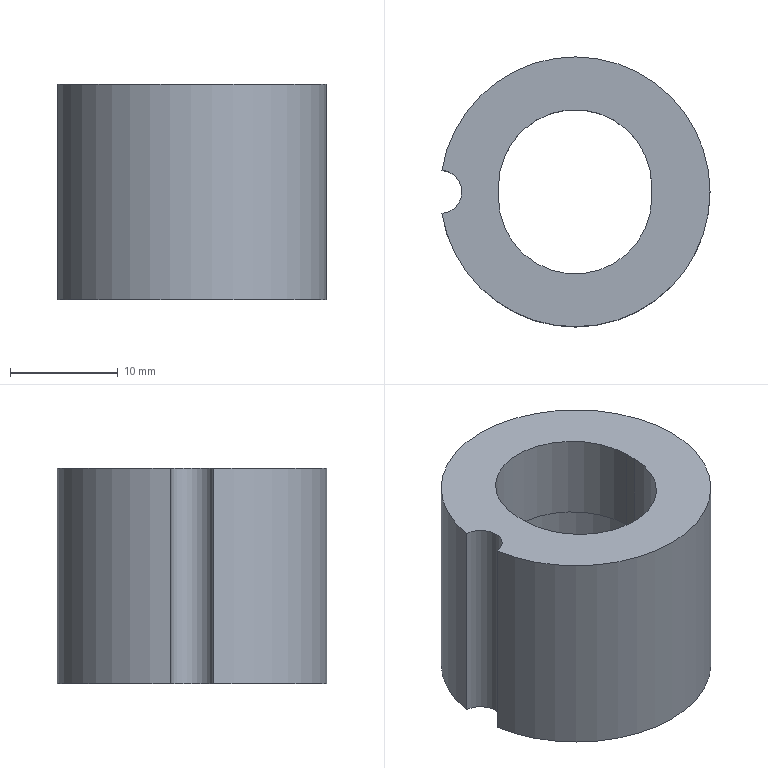Part | NX | features solid 2 | 1 solid | 10 faces | box 24.84 x 25 x 20 mm | volume 5715 mm3 | plane 5 | cylinder 5 | commonest cylinder face diameters 14.22 x2 4 x1 16.6 x1 25 x1
STEP:
#1=CARTESIAN_POINT('',(-114.371,25.823,-5.379));
#2=VERTEX_POINT('',#1);
#3=CARTESIAN_POINT('',(-114.371,21.836,-5.379));
#4=VERTEX_POINT('',#3);
#5=CARTESIAN_POINT('',(-114.531,23.83,-5.379));
#6=DIRECTION('',(0.,0.,-1.));
#7=DIRECTION('',(1.,0.,0.));
#8=AXIS2_PLACEMENT_3D('',#5,#6,#7);
#9=CIRCLE('',#8,2.);
#10=EDGE_CURVE('',#2,#4,#9,.T.);
#11=ORIENTED_EDGE('',*,*,#10,.T.);
#12=CARTESIAN_POINT('',(-102.031,23.83,-5.379));
#13=DIRECTION('',(0.,0.,1.));
#14=DIRECTION('',(-1.,0.,0.));
#15=AXIS2_PLACEMENT_3D('',#12,#13,#14);
#16=CIRCLE('',#15,12.5);
#17=EDGE_CURVE('',#2,#4,#16,.F.);
#18=ORIENTED_EDGE('',*,*,#17,.F.);
#19=EDGE_LOOP('',(#11,#18));
#20=FACE_BOUND('',#19,.T.);
#21=CARTESIAN_POINT('',(-94.921,23.33,-5.379));
#22=VERTEX_POINT('',#21);
#23=CARTESIAN_POINT('',(-109.141,23.33,-5.379));
#24=VERTEX_POINT('',#23);
#25=CARTESIAN_POINT('',(-102.031,23.33,-5.379));
#26=DIRECTION('',(0.,0.,-1.));
#27=DIRECTION('',(1.,0.,0.));
#28=AXIS2_PLACEMENT_3D('',#25,#26,#27);
#29=CIRCLE('',#28,7.11);
#30=EDGE_CURVE('',#22,#24,#29,.T.);
#31=ORIENTED_EDGE('',*,*,#30,.T.);
#32=CARTESIAN_POINT('',(-109.141,24.33,-5.379));
#33=VERTEX_POINT('',#32);
#34=CARTESIAN_POINT('',(-109.141,23.83,-5.379));
#35=DIRECTION('',(0.,1.,0.));
#36=VECTOR('',#35,1000.);
#37=LINE('',#34,#36);
#38=EDGE_CURVE('',#24,#33,#37,.T.);
#39=ORIENTED_EDGE('',*,*,#38,.T.);
#40=CARTESIAN_POINT('',(-94.921,24.33,-5.379));
#41=VERTEX_POINT('',#40);
#42=CARTESIAN_POINT('',(-102.031,24.33,-5.379));
#43=DIRECTION('',(0.,0.,-1.));
#44=DIRECTION('',(1.,0.,0.));
#45=AXIS2_PLACEMENT_3D('',#42,#43,#44);
#46=CIRCLE('',#45,7.11);
#47=EDGE_CURVE('',#33,#41,#46,.T.);
#48=ORIENTED_EDGE('',*,*,#47,.T.);
#49=CARTESIAN_POINT('',(-94.921,23.83,-5.379));
#50=DIRECTION('',(0.,-1.,0.));
#51=VECTOR('',#50,1000.);
#52=LINE('',#49,#51);
#53=EDGE_CURVE('',#41,#22,#52,.T.);
#54=ORIENTED_EDGE('',*,*,#53,.T.);
#55=EDGE_LOOP('',(#31,#39,#48,#54));
#56=FACE_BOUND('',#55,.T.);
#57=CARTESIAN_POINT('',(-102.031,23.83,-5.379));
#58=DIRECTION('',(0.,0.,1.));
#59=DIRECTION('',(-1.,0.,0.));
#60=AXIS2_PLACEMENT_3D('',#57,#58,#59);
#61=PLANE('',#60);
#62=ADVANCED_FACE('',(#20,#56),#61,.T.);
#63=CARTESIAN_POINT('',(-114.371,21.836,-25.379));
#64=VERTEX_POINT('',#63);
#65=CARTESIAN_POINT('',(-114.371,25.823,-25.379));
#66=VERTEX_POINT('',#65);
#67=CARTESIAN_POINT('',(-114.531,23.83,-25.379));
#68=DIRECTION('',(0.,0.,1.));
#69=DIRECTION('',(-1.,0.,0.));
#70=AXIS2_PLACEMENT_3D('',#67,#68,#69);
#71=CIRCLE('',#70,2.);
#72=EDGE_CURVE('',#64,#66,#71,.T.);
#73=ORIENTED_EDGE('',*,*,#72,.T.);
#74=CARTESIAN_POINT('',(-102.031,23.83,-25.379));
#75=DIRECTION('',(0.,0.,-1.));
#76=DIRECTION('',(1.,0.,0.));
#77=AXIS2_PLACEMENT_3D('',#74,#75,#76);
#78=CIRCLE('',#77,12.5);
#79=EDGE_CURVE('',#64,#66,#78,.F.);
#80=ORIENTED_EDGE('',*,*,#79,.F.);
#81=EDGE_LOOP('',(#73,#80));
#82=FACE_BOUND('',#81,.T.);
#83=CARTESIAN_POINT('',(-93.731,23.83,-25.379));
#84=VERTEX_POINT('',#83);
#85=CARTESIAN_POINT('',(-102.031,23.83,-25.379));
#86=DIRECTION('',(0.,0.,-1.));
#87=DIRECTION('',(1.,0.,0.));
#88=AXIS2_PLACEMENT_3D('',#85,#86,#87);
#89=CIRCLE('',#88,8.3);
#90=EDGE_CURVE('',#84,#84,#89,.F.);
#91=ORIENTED_EDGE('',*,*,#90,.T.);
#92=EDGE_LOOP('',(#91));
#93=FACE_BOUND('',#92,.T.);
#94=CARTESIAN_POINT('',(-102.031,23.83,-25.379));
#95=DIRECTION('',(0.,0.,-1.));
#96=DIRECTION('',(1.,0.,0.));
#97=AXIS2_PLACEMENT_3D('',#94,#95,#96);
#98=PLANE('',#97);
#99=ADVANCED_FACE('',(#82,#93),#98,.T.);
#100=CARTESIAN_POINT('',(-114.371,21.836,-15.379));
#101=DIRECTION('',(0.,0.,1.));
#102=VECTOR('',#101,1000.);
#103=LINE('',#100,#102);
#104=EDGE_CURVE('',#64,#4,#103,.T.);
#105=ORIENTED_EDGE('',*,*,#104,.F.);
#106=ORIENTED_EDGE('',*,*,#79,.T.);
#107=CARTESIAN_POINT('',(-114.371,25.823,-15.379));
#108=DIRECTION('',(0.,0.,1.));
#109=VECTOR('',#108,1000.);
#110=LINE('',#107,#109);
#111=EDGE_CURVE('',#2,#66,#110,.F.);
#112=ORIENTED_EDGE('',*,*,#111,.F.);
#113=ORIENTED_EDGE('',*,*,#17,.T.);
#114=EDGE_LOOP('',(#105,#106,#112,#113));
#115=FACE_BOUND('',#114,.T.);
#116=CARTESIAN_POINT('',(-102.031,23.83,-25.379));
#117=DIRECTION('',(0.,0.,1.));
#118=DIRECTION('',(-1.,0.,0.));
#119=AXIS2_PLACEMENT_3D('',#116,#117,#118);
#120=CYLINDRICAL_SURFACE('',#119,12.5);
#121=ADVANCED_FACE('',(#115),#120,.T.);
#122=CARTESIAN_POINT('',(-109.141,24.33,-13.379));
#123=VERTEX_POINT('',#122);
#124=CARTESIAN_POINT('',(-109.141,23.33,-13.379));
#125=VERTEX_POINT('',#124);
#126=CARTESIAN_POINT('',(-109.141,23.83,-13.379));
#127=DIRECTION('',(0.,-1.,0.));
#128=VECTOR('',#127,1000.);
#129=LINE('',#126,#128);
#130=EDGE_CURVE('',#123,#125,#129,.T.);
#131=ORIENTED_EDGE('',*,*,#130,.T.);
#132=CARTESIAN_POINT('',(-94.921,23.33,-13.379));
#133=VERTEX_POINT('',#132);
#134=CARTESIAN_POINT('',(-102.031,23.33,-13.379));
#135=DIRECTION('',(0.,0.,1.));
#136=DIRECTION('',(-1.,0.,0.));
#137=AXIS2_PLACEMENT_3D('',#134,#135,#136);
#138=CIRCLE('',#137,7.11);
#139=EDGE_CURVE('',#125,#133,#138,.T.);
#140=ORIENTED_EDGE('',*,*,#139,.T.);
#141=CARTESIAN_POINT('',(-94.921,24.33,-13.379));
#142=VERTEX_POINT('',#141);
#143=CARTESIAN_POINT('',(-94.921,23.83,-13.379));
#144=DIRECTION('',(0.,1.,0.));
#145=VECTOR('',#144,1000.);
#146=LINE('',#143,#145);
#147=EDGE_CURVE('',#133,#142,#146,.T.);
#148=ORIENTED_EDGE('',*,*,#147,.T.);
#149=CARTESIAN_POINT('',(-102.031,24.33,-13.379));
#150=DIRECTION('',(0.,0.,1.));
#151=DIRECTION('',(-1.,0.,0.));
#152=AXIS2_PLACEMENT_3D('',#149,#150,#151);
#153=CIRCLE('',#152,7.11);
#154=EDGE_CURVE('',#142,#123,#153,.T.);
#155=ORIENTED_EDGE('',*,*,#154,.T.);
#156=EDGE_LOOP('',(#131,#140,#148,#155));
#157=FACE_BOUND('',#156,.T.);
#158=CARTESIAN_POINT('',(-110.331,23.83,-13.379));
#159=VERTEX_POINT('',#158);
#160=CARTESIAN_POINT('',(-102.031,23.83,-13.379));
#161=DIRECTION('',(0.,0.,1.));
#162=DIRECTION('',(-1.,0.,0.));
#163=AXIS2_PLACEMENT_3D('',#160,#161,#162);
#164=CIRCLE('',#163,8.3);
#165=EDGE_CURVE('',#159,#159,#164,.F.);
#166=ORIENTED_EDGE('',*,*,#165,.T.);
#167=EDGE_LOOP('',(#166));
#168=FACE_BOUND('',#167,.T.);
#169=CARTESIAN_POINT('',(-102.031,23.83,-13.379));
#170=DIRECTION('',(0.,0.,1.));
#171=DIRECTION('',(-1.,0.,0.));
#172=AXIS2_PLACEMENT_3D('',#169,#170,#171);
#173=PLANE('',#172);
#174=ADVANCED_FACE('',(#157,#168),#173,.F.);
#175=ORIENTED_EDGE('',*,*,#165,.F.);
#176=EDGE_LOOP('',(#175));
#177=FACE_BOUND('',#176,.T.);
#178=ORIENTED_EDGE('',*,*,#90,.F.);
#179=EDGE_LOOP('',(#178));
#180=FACE_BOUND('',#179,.T.);
#181=CARTESIAN_POINT('',(-102.031,23.83,-25.379));
#182=DIRECTION('',(0.,0.,1.));
#183=DIRECTION('',(-1.,0.,0.));
#184=AXIS2_PLACEMENT_3D('',#181,#182,#183);
#185=CYLINDRICAL_SURFACE('',#184,8.3);
#186=ADVANCED_FACE('',(#177,#180),#185,.F.);
#187=CARTESIAN_POINT('',(-94.921,24.33,-13.379));
#188=DIRECTION('',(0.,0.,1.));
#189=VECTOR('',#188,1000.);
#190=LINE('',#187,#189);
#191=EDGE_CURVE('',#142,#41,#190,.T.);
#192=ORIENTED_EDGE('',*,*,#191,.F.);
#193=ORIENTED_EDGE('',*,*,#147,.F.);
#194=CARTESIAN_POINT('',(-94.921,23.33,-13.379));
#195=DIRECTION('',(0.,0.,1.));
#196=VECTOR('',#195,1000.);
#197=LINE('',#194,#196);
#198=EDGE_CURVE('',#133,#22,#197,.T.);
#199=ORIENTED_EDGE('',*,*,#198,.T.);
#200=ORIENTED_EDGE('',*,*,#53,.F.);
#201=EDGE_LOOP('',(#192,#193,#199,#200));
#202=FACE_BOUND('',#201,.T.);
#203=CARTESIAN_POINT('',(-94.921,23.83,-13.379));
#204=DIRECTION('',(1.,0.,0.));
#205=DIRECTION('',(0.,0.,1.));
#206=AXIS2_PLACEMENT_3D('',#203,#204,#205);
#207=PLANE('',#206);
#208=ADVANCED_FACE('',(#202),#207,.F.);
#209=ORIENTED_EDGE('',*,*,#130,.F.);
#210=CARTESIAN_POINT('',(-109.141,24.33,-13.379));
#211=DIRECTION('',(0.,0.,1.));
#212=VECTOR('',#211,1000.);
#213=LINE('',#210,#212);
#214=EDGE_CURVE('',#123,#33,#213,.T.);
#215=ORIENTED_EDGE('',*,*,#214,.T.);
#216=ORIENTED_EDGE('',*,*,#38,.F.);
#217=CARTESIAN_POINT('',(-109.141,23.33,-13.379));
#218=DIRECTION('',(0.,0.,1.));
#219=VECTOR('',#218,1000.);
#220=LINE('',#217,#219);
#221=EDGE_CURVE('',#125,#24,#220,.T.);
#222=ORIENTED_EDGE('',*,*,#221,.F.);
#223=EDGE_LOOP('',(#209,#215,#216,#222));
#224=FACE_BOUND('',#223,.T.);
#225=CARTESIAN_POINT('',(-109.141,23.83,-13.379));
#226=DIRECTION('',(-1.,0.,0.));
#227=DIRECTION('',(0.,0.,-1.));
#228=AXIS2_PLACEMENT_3D('',#225,#226,#227);
#229=PLANE('',#228);
#230=ADVANCED_FACE('',(#224),#229,.F.);
#231=ORIENTED_EDGE('',*,*,#191,.T.);
#232=ORIENTED_EDGE('',*,*,#47,.F.);
#233=ORIENTED_EDGE('',*,*,#214,.F.);
#234=ORIENTED_EDGE('',*,*,#154,.F.);
#235=EDGE_LOOP('',(#231,#232,#233,#234));
#236=FACE_BOUND('',#235,.T.);
#237=CARTESIAN_POINT('',(-102.031,24.33,-13.379));
#238=DIRECTION('',(0.,0.,1.));
#239=DIRECTION('',(-1.,0.,0.));
#240=AXIS2_PLACEMENT_3D('',#237,#238,#239);
#241=CYLINDRICAL_SURFACE('',#240,7.11);
#242=ADVANCED_FACE('',(#236),#241,.F.);
#243=ORIENTED_EDGE('',*,*,#139,.F.);
#244=ORIENTED_EDGE('',*,*,#221,.T.);
#245=ORIENTED_EDGE('',*,*,#30,.F.);
#246=ORIENTED_EDGE('',*,*,#198,.F.);
#247=EDGE_LOOP('',(#243,#244,#245,#246));
#248=FACE_BOUND('',#247,.T.);
#249=CARTESIAN_POINT('',(-102.031,23.33,-13.379));
#250=DIRECTION('',(0.,0.,1.));
#251=DIRECTION('',(-1.,0.,0.));
#252=AXIS2_PLACEMENT_3D('',#249,#250,#251);
#253=CYLINDRICAL_SURFACE('',#252,7.11);
#254=ADVANCED_FACE('',(#248),#253,.F.);
#255=ORIENTED_EDGE('',*,*,#104,.T.);
#256=ORIENTED_EDGE('',*,*,#10,.F.);
#257=ORIENTED_EDGE('',*,*,#111,.T.);
#258=ORIENTED_EDGE('',*,*,#72,.F.);
#259=EDGE_LOOP('',(#255,#256,#257,#258));
#260=FACE_BOUND('',#259,.T.);
#261=CARTESIAN_POINT('',(-114.531,23.83,-25.379));
#262=DIRECTION('',(0.,0.,1.));
#263=DIRECTION('',(-1.,0.,0.));
#264=AXIS2_PLACEMENT_3D('',#261,#262,#263);
#265=CYLINDRICAL_SURFACE('',#264,2.);
#266=ADVANCED_FACE('',(#260),#265,.F.);
#267=CLOSED_SHELL('',(#62,#99,#121,#174,#186,#208,#230,#242,#254,#266));
#268=MANIFOLD_SOLID_BREP('',#267);
#269=(LENGTH_UNIT()NAMED_UNIT(*)SI_UNIT(.MILLI.,.METRE.));
#270=UNCERTAINTY_MEASURE_WITH_UNIT(LENGTH_MEASURE(0.00001),#269,'','');
#271=(NAMED_UNIT(*)PLANE_ANGLE_UNIT()SI_UNIT($,.RADIAN.));
#272=(NAMED_UNIT(*)SI_UNIT($,.STERADIAN.)SOLID_ANGLE_UNIT());
#273=(GEOMETRIC_REPRESENTATION_CONTEXT(3)GLOBAL_UNCERTAINTY_ASSIGNED_CONTEXT((#270))GLOBAL_UNIT_ASSIGNED_CONTEXT((#269,#271,#272))REPRESENTATION_CONTEXT('',''));
#274=ADVANCED_BREP_SHAPE_REPRESENTATION('',(#268),#273);